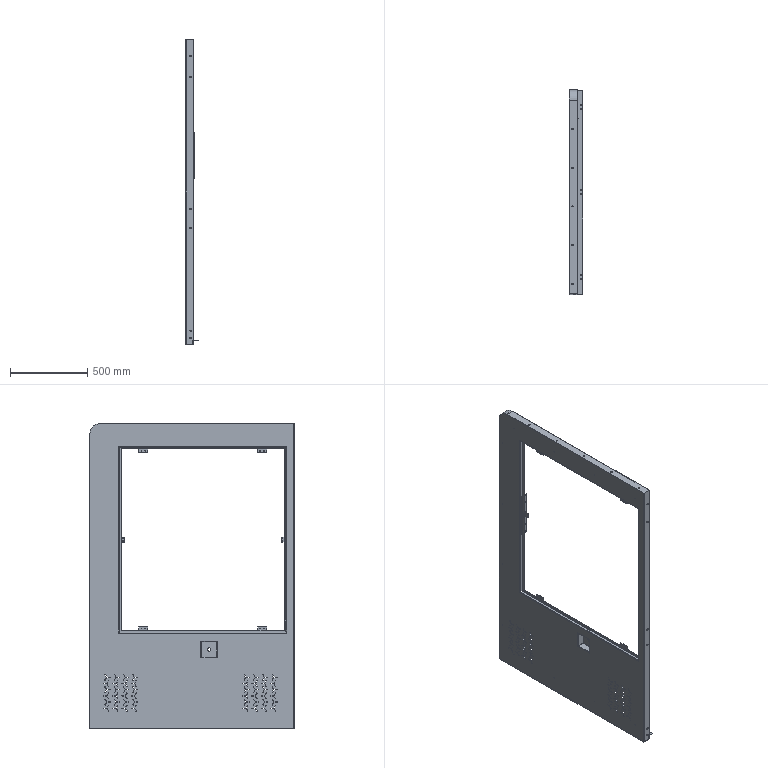Part | NX | features BREP 4 | 4 solids | 843 faces | box 84.5 x 1322 x 1970 mm | volume 2847366 mm3 | plane 476 | cylinder 343 | spline 24 | commonest cylinder face diameters 3 x192 5 x52 7 x36 4 x24 5.5 x16 6 x15